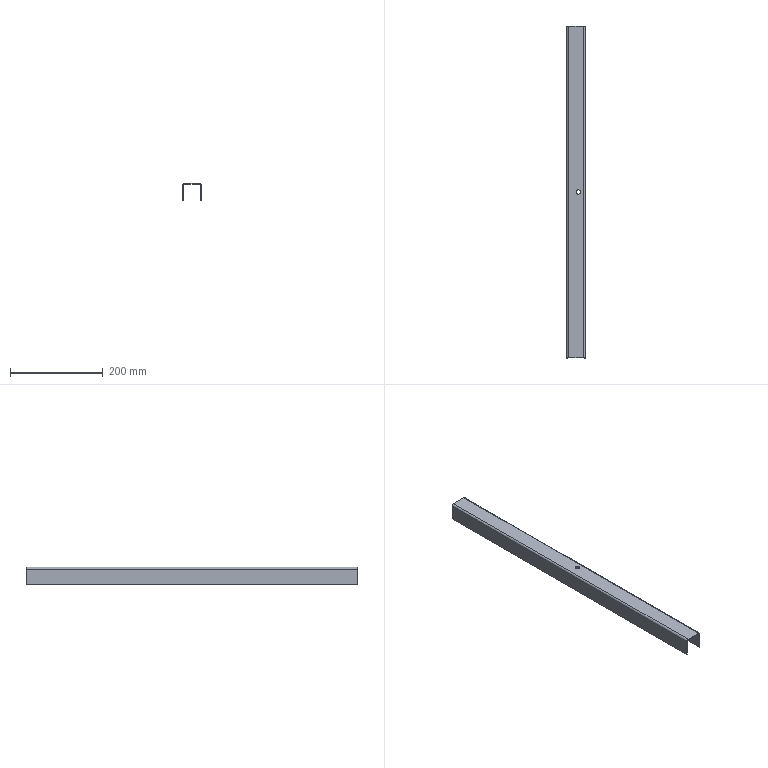Part | NX | features solid 2 | 1 solid | 16 faces | box 40 x 717 x 38 mm | volume 156782 mm3 | plane 10 | cylinder 6 | commonest cylinder face diameters 4 x2 8 x2 9.2 x2
STEP:
#1=CARTESIAN_POINT('',(-836.,-1113.1,1293.));
#2=VERTEX_POINT('',#1);
#3=CARTESIAN_POINT('',(-836.,-1113.1,1295.));
#4=VERTEX_POINT('',#3);
#5=CARTESIAN_POINT('',(-836.,-1113.1,575.88));
#6=DIRECTION('',(0.,0.,1.));
#7=VECTOR('',#6,1000.);
#8=LINE('',#5,#7);
#9=EDGE_CURVE('',#2,#4,#8,.T.);
#10=ORIENTED_EDGE('',*,*,#9,.F.);
#11=CARTESIAN_POINT('',(-836.,-1103.9,1293.));
#12=VERTEX_POINT('',#11);
#13=CARTESIAN_POINT('',(-836.,-1108.5,1293.));
#14=DIRECTION('',(0.,0.,-1.));
#15=DIRECTION('',(0.,-1.,0.));
#16=AXIS2_PLACEMENT_3D('',#13,#14,#15);
#17=CIRCLE('',#16,4.6);
#18=EDGE_CURVE('',#2,#12,#17,.T.);
#19=ORIENTED_EDGE('',*,*,#18,.T.);
#20=CARTESIAN_POINT('',(-836.,-1103.9,1295.));
#21=VERTEX_POINT('',#20);
#22=CARTESIAN_POINT('',(-836.,-1103.9,575.88));
#23=DIRECTION('',(0.,0.,1.));
#24=VECTOR('',#23,1000.);
#25=LINE('',#22,#24);
#26=EDGE_CURVE('',#21,#12,#25,.F.);
#27=ORIENTED_EDGE('',*,*,#26,.F.);
#28=CARTESIAN_POINT('',(-836.,-1108.5,1295.));
#29=DIRECTION('',(0.,0.,1.));
#30=DIRECTION('',(0.,-1.,0.));
#31=AXIS2_PLACEMENT_3D('',#28,#29,#30);
#32=CIRCLE('',#31,4.6);
#33=EDGE_CURVE('',#21,#4,#32,.T.);
#34=ORIENTED_EDGE('',*,*,#33,.T.);
#35=EDGE_LOOP('',(#10,#19,#27,#34));
#36=FACE_BOUND('',#35,.T.);
#37=CARTESIAN_POINT('',(-836.,-1108.5,575.88));
#38=DIRECTION('',(0.,0.,1.));
#39=DIRECTION('',(0.,1.,0.));
#40=AXIS2_PLACEMENT_3D('',#37,#38,#39);
#41=CYLINDRICAL_SURFACE('',#40,4.6);
#42=ADVANCED_FACE('',(#36),#41,.F.);
#43=CARTESIAN_POINT('',(-821.,-1467.,1291.));
#44=VERTEX_POINT('',#43);
#45=CARTESIAN_POINT('',(-821.,-1467.,1257.));
#46=VERTEX_POINT('',#45);
#47=CARTESIAN_POINT('',(-821.,-1467.,1295.));
#48=DIRECTION('',(0.,0.,-1.));
#49=VECTOR('',#48,1000.);
#50=LINE('',#47,#49);
#51=EDGE_CURVE('',#44,#46,#50,.T.);
#52=ORIENTED_EDGE('',*,*,#51,.T.);
#53=CARTESIAN_POINT('',(-821.,-750.,1257.));
#54=VERTEX_POINT('',#53);
#55=CARTESIAN_POINT('',(-821.,-750.,1257.));
#56=DIRECTION('',(0.,-1.,0.));
#57=VECTOR('',#56,1000.);
#58=LINE('',#55,#57);
#59=EDGE_CURVE('',#54,#46,#58,.T.);
#60=ORIENTED_EDGE('',*,*,#59,.F.);
#61=CARTESIAN_POINT('',(-821.,-750.,1291.));
#62=VERTEX_POINT('',#61);
#63=CARTESIAN_POINT('',(-821.,-750.,1295.));
#64=DIRECTION('',(0.,0.,-1.));
#65=VECTOR('',#64,1000.);
#66=LINE('',#63,#65);
#67=EDGE_CURVE('',#62,#54,#66,.T.);
#68=ORIENTED_EDGE('',*,*,#67,.F.);
#69=CARTESIAN_POINT('',(-821.,-750.,1291.));
#70=DIRECTION('',(0.,-1.,0.));
#71=VECTOR('',#70,1000.);
#72=LINE('',#69,#71);
#73=EDGE_CURVE('',#62,#44,#72,.T.);
#74=ORIENTED_EDGE('',*,*,#73,.T.);
#75=EDGE_LOOP('',(#52,#60,#68,#74));
#76=FACE_BOUND('',#75,.T.);
#77=CARTESIAN_POINT('',(-821.,-750.,1295.));
#78=DIRECTION('',(-1.,0.,0.));
#79=DIRECTION('',(0.,0.,1.));
#80=AXIS2_PLACEMENT_3D('',#77,#78,#79);
#81=PLANE('',#80);
#82=ADVANCED_FACE('',(#76),#81,.F.);
#83=CARTESIAN_POINT('',(-825.,-1467.,1295.));
#84=VERTEX_POINT('',#83);
#85=CARTESIAN_POINT('',(-825.,-1467.,1291.));
#86=DIRECTION('',(0.,1.,0.));
#87=DIRECTION('',(-1.,0.,0.));
#88=AXIS2_PLACEMENT_3D('',#85,#86,#87);
#89=CIRCLE('',#88,4.);
#90=EDGE_CURVE('',#84,#44,#89,.T.);
#91=ORIENTED_EDGE('',*,*,#90,.T.);
#92=ORIENTED_EDGE('',*,*,#73,.F.);
#93=CARTESIAN_POINT('',(-825.,-750.,1295.));
#94=VERTEX_POINT('',#93);
#95=CARTESIAN_POINT('',(-825.,-750.,1291.));
#96=DIRECTION('',(0.,1.,0.));
#97=DIRECTION('',(-1.,0.,0.));
#98=AXIS2_PLACEMENT_3D('',#95,#96,#97);
#99=CIRCLE('',#98,4.);
#100=EDGE_CURVE('',#94,#62,#99,.T.);
#101=ORIENTED_EDGE('',*,*,#100,.F.);
#102=CARTESIAN_POINT('',(-825.,-750.,1295.));
#103=DIRECTION('',(0.,-1.,0.));
#104=VECTOR('',#103,1000.);
#105=LINE('',#102,#104);
#106=EDGE_CURVE('',#94,#84,#105,.T.);
#107=ORIENTED_EDGE('',*,*,#106,.T.);
#108=EDGE_LOOP('',(#91,#92,#101,#107));
#109=FACE_BOUND('',#108,.T.);
#110=CARTESIAN_POINT('',(-825.,-750.,1291.));
#111=DIRECTION('',(0.,-1.,0.));
#112=DIRECTION('',(0.,0.,1.));
#113=AXIS2_PLACEMENT_3D('',#110,#111,#112);
#114=CYLINDRICAL_SURFACE('',#113,4.);
#115=ADVANCED_FACE('',(#109),#114,.T.);
#116=ORIENTED_EDGE('',*,*,#33,.F.);
#117=CARTESIAN_POINT('',(-836.,-1108.5,1295.));
#118=DIRECTION('',(0.,0.,1.));
#119=DIRECTION('',(0.,-1.,0.));
#120=AXIS2_PLACEMENT_3D('',#117,#118,#119);
#121=CIRCLE('',#120,4.6);
#122=EDGE_CURVE('',#4,#21,#121,.T.);
#123=ORIENTED_EDGE('',*,*,#122,.F.);
#124=EDGE_LOOP('',(#116,#123));
#125=FACE_BOUND('',#124,.T.);
#126=CARTESIAN_POINT('',(-857.,-1467.,1295.));
#127=VERTEX_POINT('',#126);
#128=CARTESIAN_POINT('',(-861.,-1467.,1295.));
#129=DIRECTION('',(1.,0.,0.));
#130=VECTOR('',#129,1000.);
#131=LINE('',#128,#130);
#132=EDGE_CURVE('',#127,#84,#131,.T.);
#133=ORIENTED_EDGE('',*,*,#132,.T.);
#134=ORIENTED_EDGE('',*,*,#106,.F.);
#135=CARTESIAN_POINT('',(-857.,-750.,1295.));
#136=VERTEX_POINT('',#135);
#137=CARTESIAN_POINT('',(-861.,-750.,1295.));
#138=DIRECTION('',(1.,0.,0.));
#139=VECTOR('',#138,1000.);
#140=LINE('',#137,#139);
#141=EDGE_CURVE('',#136,#94,#140,.T.);
#142=ORIENTED_EDGE('',*,*,#141,.F.);
#143=CARTESIAN_POINT('',(-857.,-750.,1295.));
#144=DIRECTION('',(0.,-1.,0.));
#145=VECTOR('',#144,1000.);
#146=LINE('',#143,#145);
#147=EDGE_CURVE('',#136,#127,#146,.T.);
#148=ORIENTED_EDGE('',*,*,#147,.T.);
#149=EDGE_LOOP('',(#133,#134,#142,#148));
#150=FACE_BOUND('',#149,.T.);
#151=CARTESIAN_POINT('',(-861.,-750.,1295.));
#152=DIRECTION('',(0.,0.,-1.));
#153=DIRECTION('',(0.,-1.,0.));
#154=AXIS2_PLACEMENT_3D('',#151,#152,#153);
#155=PLANE('',#154);
#156=ADVANCED_FACE('',(#125,#150),#155,.F.);
#157=CARTESIAN_POINT('',(-861.,-1467.,1291.));
#158=VERTEX_POINT('',#157);
#159=CARTESIAN_POINT('',(-857.,-1467.,1291.));
#160=DIRECTION('',(0.,1.,0.));
#161=DIRECTION('',(-1.,0.,0.));
#162=AXIS2_PLACEMENT_3D('',#159,#160,#161);
#163=CIRCLE('',#162,4.);
#164=EDGE_CURVE('',#158,#127,#163,.T.);
#165=ORIENTED_EDGE('',*,*,#164,.T.);
#166=ORIENTED_EDGE('',*,*,#147,.F.);
#167=CARTESIAN_POINT('',(-861.,-750.,1291.));
#168=VERTEX_POINT('',#167);
#169=CARTESIAN_POINT('',(-857.,-750.,1291.));
#170=DIRECTION('',(0.,1.,0.));
#171=DIRECTION('',(-1.,0.,0.));
#172=AXIS2_PLACEMENT_3D('',#169,#170,#171);
#173=CIRCLE('',#172,4.);
#174=EDGE_CURVE('',#168,#136,#173,.T.);
#175=ORIENTED_EDGE('',*,*,#174,.F.);
#176=CARTESIAN_POINT('',(-861.,-750.,1291.));
#177=DIRECTION('',(0.,-1.,0.));
#178=VECTOR('',#177,1000.);
#179=LINE('',#176,#178);
#180=EDGE_CURVE('',#168,#158,#179,.T.);
#181=ORIENTED_EDGE('',*,*,#180,.T.);
#182=EDGE_LOOP('',(#165,#166,#175,#181));
#183=FACE_BOUND('',#182,.T.);
#184=CARTESIAN_POINT('',(-857.,-750.,1291.));
#185=DIRECTION('',(0.,-1.,0.));
#186=DIRECTION('',(0.,0.,1.));
#187=AXIS2_PLACEMENT_3D('',#184,#185,#186);
#188=CYLINDRICAL_SURFACE('',#187,4.);
#189=ADVANCED_FACE('',(#183),#188,.T.);
#190=CARTESIAN_POINT('',(-861.,-1467.,1257.));
#191=VERTEX_POINT('',#190);
#192=CARTESIAN_POINT('',(-861.,-1467.,1257.));
#193=DIRECTION('',(0.,0.,1.));
#194=VECTOR('',#193,1000.);
#195=LINE('',#192,#194);
#196=EDGE_CURVE('',#191,#158,#195,.T.);
#197=ORIENTED_EDGE('',*,*,#196,.T.);
#198=ORIENTED_EDGE('',*,*,#180,.F.);
#199=CARTESIAN_POINT('',(-861.,-750.,1257.));
#200=VERTEX_POINT('',#199);
#201=CARTESIAN_POINT('',(-861.,-750.,1257.));
#202=DIRECTION('',(0.,0.,1.));
#203=VECTOR('',#202,1000.);
#204=LINE('',#201,#203);
#205=EDGE_CURVE('',#200,#168,#204,.T.);
#206=ORIENTED_EDGE('',*,*,#205,.F.);
#207=CARTESIAN_POINT('',(-861.,-750.,1257.));
#208=DIRECTION('',(0.,-1.,0.));
#209=VECTOR('',#208,1000.);
#210=LINE('',#207,#209);
#211=EDGE_CURVE('',#200,#191,#210,.T.);
#212=ORIENTED_EDGE('',*,*,#211,.T.);
#213=EDGE_LOOP('',(#197,#198,#206,#212));
#214=FACE_BOUND('',#213,.T.);
#215=CARTESIAN_POINT('',(-861.,-750.,1257.));
#216=DIRECTION('',(1.,0.,0.));
#217=DIRECTION('',(0.,0.,1.));
#218=AXIS2_PLACEMENT_3D('',#215,#216,#217);
#219=PLANE('',#218);
#220=ADVANCED_FACE('',(#214),#219,.F.);
#221=CARTESIAN_POINT('',(-823.,-1467.,1291.));
#222=VERTEX_POINT('',#221);
#223=CARTESIAN_POINT('',(-823.,-1467.,1257.));
#224=VERTEX_POINT('',#223);
#225=CARTESIAN_POINT('',(-823.,-1467.,1295.));
#226=DIRECTION('',(0.,0.,-1.));
#227=VECTOR('',#226,1000.);
#228=LINE('',#225,#227);
#229=EDGE_CURVE('',#222,#224,#228,.T.);
#230=ORIENTED_EDGE('',*,*,#229,.F.);
#231=CARTESIAN_POINT('',(-823.,-750.,1291.));
#232=VERTEX_POINT('',#231);
#233=CARTESIAN_POINT('',(-823.,-750.,1291.));
#234=DIRECTION('',(0.,-1.,0.));
#235=VECTOR('',#234,1000.);
#236=LINE('',#233,#235);
#237=EDGE_CURVE('',#232,#222,#236,.T.);
#238=ORIENTED_EDGE('',*,*,#237,.F.);
#239=CARTESIAN_POINT('',(-823.,-750.,1257.));
#240=VERTEX_POINT('',#239);
#241=CARTESIAN_POINT('',(-823.,-750.,1295.));
#242=DIRECTION('',(0.,0.,-1.));
#243=VECTOR('',#242,1000.);
#244=LINE('',#241,#243);
#245=EDGE_CURVE('',#232,#240,#244,.T.);
#246=ORIENTED_EDGE('',*,*,#245,.T.);
#247=CARTESIAN_POINT('',(-823.,-750.,1257.));
#248=DIRECTION('',(0.,-1.,0.));
#249=VECTOR('',#248,1000.);
#250=LINE('',#247,#249);
#251=EDGE_CURVE('',#240,#224,#250,.T.);
#252=ORIENTED_EDGE('',*,*,#251,.T.);
#253=EDGE_LOOP('',(#230,#238,#246,#252));
#254=FACE_BOUND('',#253,.T.);
#255=CARTESIAN_POINT('',(-823.,-750.,1295.));
#256=DIRECTION('',(-1.,0.,0.));
#257=DIRECTION('',(0.,0.,1.));
#258=AXIS2_PLACEMENT_3D('',#255,#256,#257);
#259=PLANE('',#258);
#260=ADVANCED_FACE('',(#254),#259,.T.);
#261=CARTESIAN_POINT('',(-825.,-1467.,1293.));
#262=VERTEX_POINT('',#261);
#263=CARTESIAN_POINT('',(-825.,-1467.,1291.));
#264=DIRECTION('',(0.,1.,0.));
#265=DIRECTION('',(0.,0.,1.));
#266=AXIS2_PLACEMENT_3D('',#263,#264,#265);
#267=CIRCLE('',#266,2.);
#268=EDGE_CURVE('',#262,#222,#267,.T.);
#269=ORIENTED_EDGE('',*,*,#268,.F.);
#270=CARTESIAN_POINT('',(-825.,-750.,1293.));
#271=VERTEX_POINT('',#270);
#272=CARTESIAN_POINT('',(-825.,-750.,1293.));
#273=DIRECTION('',(0.,-1.,0.));
#274=VECTOR('',#273,1000.);
#275=LINE('',#272,#274);
#276=EDGE_CURVE('',#271,#262,#275,.T.);
#277=ORIENTED_EDGE('',*,*,#276,.F.);
#278=CARTESIAN_POINT('',(-825.,-750.,1291.));
#279=DIRECTION('',(0.,1.,0.));
#280=DIRECTION('',(0.,0.,1.));
#281=AXIS2_PLACEMENT_3D('',#278,#279,#280);
#282=CIRCLE('',#281,2.);
#283=EDGE_CURVE('',#271,#232,#282,.T.);
#284=ORIENTED_EDGE('',*,*,#283,.T.);
#285=ORIENTED_EDGE('',*,*,#237,.T.);
#286=EDGE_LOOP('',(#269,#277,#284,#285));
#287=FACE_BOUND('',#286,.T.);
#288=CARTESIAN_POINT('',(-825.,-750.,1291.));
#289=DIRECTION('',(0.,-1.,0.));
#290=DIRECTION('',(0.,0.,1.));
#291=AXIS2_PLACEMENT_3D('',#288,#289,#290);
#292=CYLINDRICAL_SURFACE('',#291,2.);
#293=ADVANCED_FACE('',(#287),#292,.F.);
#294=CARTESIAN_POINT('',(-836.,-1108.5,1293.));
#295=DIRECTION('',(0.,0.,-1.));
#296=DIRECTION('',(0.,-1.,0.));
#297=AXIS2_PLACEMENT_3D('',#294,#295,#296);
#298=CIRCLE('',#297,4.6);
#299=EDGE_CURVE('',#12,#2,#298,.T.);
#300=ORIENTED_EDGE('',*,*,#299,.F.);
#301=ORIENTED_EDGE('',*,*,#18,.F.);
#302=EDGE_LOOP('',(#300,#301));
#303=FACE_BOUND('',#302,.T.);
#304=CARTESIAN_POINT('',(-857.,-1467.,1293.));
#305=VERTEX_POINT('',#304);
#306=CARTESIAN_POINT('',(-861.,-1467.,1293.));
#307=DIRECTION('',(1.,0.,0.));
#308=VECTOR('',#307,1000.);
#309=LINE('',#306,#308);
#310=EDGE_CURVE('',#305,#262,#309,.T.);
#311=ORIENTED_EDGE('',*,*,#310,.F.);
#312=CARTESIAN_POINT('',(-857.,-750.,1293.));
#313=VERTEX_POINT('',#312);
#314=CARTESIAN_POINT('',(-857.,-750.,1293.));
#315=DIRECTION('',(0.,-1.,0.));
#316=VECTOR('',#315,1000.);
#317=LINE('',#314,#316);
#318=EDGE_CURVE('',#313,#305,#317,.T.);
#319=ORIENTED_EDGE('',*,*,#318,.F.);
#320=CARTESIAN_POINT('',(-861.,-750.,1293.));
#321=DIRECTION('',(1.,0.,0.));
#322=VECTOR('',#321,1000.);
#323=LINE('',#320,#322);
#324=EDGE_CURVE('',#313,#271,#323,.T.);
#325=ORIENTED_EDGE('',*,*,#324,.T.);
#326=ORIENTED_EDGE('',*,*,#276,.T.);
#327=EDGE_LOOP('',(#311,#319,#325,#326));
#328=FACE_BOUND('',#327,.T.);
#329=CARTESIAN_POINT('',(-861.,-750.,1293.));
#330=DIRECTION('',(0.,0.,-1.));
#331=DIRECTION('',(0.,-1.,0.));
#332=AXIS2_PLACEMENT_3D('',#329,#330,#331);
#333=PLANE('',#332);
#334=ADVANCED_FACE('',(#303,#328),#333,.T.);
#335=CARTESIAN_POINT('',(-859.,-1467.,1291.));
#336=VERTEX_POINT('',#335);
#337=CARTESIAN_POINT('',(-857.,-1467.,1291.));
#338=DIRECTION('',(0.,1.,0.));
#339=DIRECTION('',(0.,0.,1.));
#340=AXIS2_PLACEMENT_3D('',#337,#338,#339);
#341=CIRCLE('',#340,2.);
#342=EDGE_CURVE('',#336,#305,#341,.T.);
#343=ORIENTED_EDGE('',*,*,#342,.F.);
#344=CARTESIAN_POINT('',(-859.,-750.,1291.));
#345=VERTEX_POINT('',#344);
#346=CARTESIAN_POINT('',(-859.,-750.,1291.));
#347=DIRECTION('',(0.,-1.,0.));
#348=VECTOR('',#347,1000.);
#349=LINE('',#346,#348);
#350=EDGE_CURVE('',#345,#336,#349,.T.);
#351=ORIENTED_EDGE('',*,*,#350,.F.);
#352=CARTESIAN_POINT('',(-857.,-750.,1291.));
#353=DIRECTION('',(0.,1.,0.));
#354=DIRECTION('',(0.,0.,1.));
#355=AXIS2_PLACEMENT_3D('',#352,#353,#354);
#356=CIRCLE('',#355,2.);
#357=EDGE_CURVE('',#345,#313,#356,.T.);
#358=ORIENTED_EDGE('',*,*,#357,.T.);
#359=ORIENTED_EDGE('',*,*,#318,.T.);
#360=EDGE_LOOP('',(#343,#351,#358,#359));
#361=FACE_BOUND('',#360,.T.);
#362=CARTESIAN_POINT('',(-857.,-750.,1291.));
#363=DIRECTION('',(0.,-1.,0.));
#364=DIRECTION('',(0.,0.,1.));
#365=AXIS2_PLACEMENT_3D('',#362,#363,#364);
#366=CYLINDRICAL_SURFACE('',#365,2.);
#367=ADVANCED_FACE('',(#361),#366,.F.);
#368=CARTESIAN_POINT('',(-859.,-1467.,1257.));
#369=VERTEX_POINT('',#368);
#370=CARTESIAN_POINT('',(-859.,-1467.,1257.));
#371=DIRECTION('',(0.,0.,1.));
#372=VECTOR('',#371,1000.);
#373=LINE('',#370,#372);
#374=EDGE_CURVE('',#369,#336,#373,.T.);
#375=ORIENTED_EDGE('',*,*,#374,.F.);
#376=CARTESIAN_POINT('',(-859.,-750.,1257.));
#377=VERTEX_POINT('',#376);
#378=CARTESIAN_POINT('',(-859.,-750.,1257.));
#379=DIRECTION('',(0.,-1.,0.));
#380=VECTOR('',#379,1000.);
#381=LINE('',#378,#380);
#382=EDGE_CURVE('',#377,#369,#381,.T.);
#383=ORIENTED_EDGE('',*,*,#382,.F.);
#384=CARTESIAN_POINT('',(-859.,-750.,1257.));
#385=DIRECTION('',(0.,0.,1.));
#386=VECTOR('',#385,1000.);
#387=LINE('',#384,#386);
#388=EDGE_CURVE('',#377,#345,#387,.T.);
#389=ORIENTED_EDGE('',*,*,#388,.T.);
#390=ORIENTED_EDGE('',*,*,#350,.T.);
#391=EDGE_LOOP('',(#375,#383,#389,#390));
#392=FACE_BOUND('',#391,.T.);
#393=CARTESIAN_POINT('',(-859.,-750.,1257.));
#394=DIRECTION('',(1.,0.,0.));
#395=DIRECTION('',(0.,0.,1.));
#396=AXIS2_PLACEMENT_3D('',#393,#394,#395);
#397=PLANE('',#396);
#398=ADVANCED_FACE('',(#392),#397,.T.);
#399=ORIENTED_EDGE('',*,*,#211,.F.);
#400=CARTESIAN_POINT('',(-861.,-750.,1257.));
#401=DIRECTION('',(1.,0.,0.));
#402=VECTOR('',#401,1000.);
#403=LINE('',#400,#402);
#404=EDGE_CURVE('',#200,#377,#403,.T.);
#405=ORIENTED_EDGE('',*,*,#404,.T.);
#406=ORIENTED_EDGE('',*,*,#382,.T.);
#407=CARTESIAN_POINT('',(-861.,-1467.,1257.));
#408=DIRECTION('',(1.,0.,0.));
#409=VECTOR('',#408,1000.);
#410=LINE('',#407,#409);
#411=EDGE_CURVE('',#191,#369,#410,.T.);
#412=ORIENTED_EDGE('',*,*,#411,.F.);
#413=EDGE_LOOP('',(#399,#405,#406,#412));
#414=FACE_BOUND('',#413,.T.);
#415=CARTESIAN_POINT('',(-861.,-750.,1257.));
#416=DIRECTION('',(0.,0.,1.));
#417=DIRECTION('',(1.,0.,0.));
#418=AXIS2_PLACEMENT_3D('',#415,#416,#417);
#419=PLANE('',#418);
#420=ADVANCED_FACE('',(#414),#419,.F.);
#421=ORIENTED_EDGE('',*,*,#374,.T.);
#422=ORIENTED_EDGE('',*,*,#342,.T.);
#423=ORIENTED_EDGE('',*,*,#310,.T.);
#424=ORIENTED_EDGE('',*,*,#268,.T.);
#425=ORIENTED_EDGE('',*,*,#229,.T.);
#426=CARTESIAN_POINT('',(-821.,-1467.,1257.));
#427=DIRECTION('',(-1.,0.,0.));
#428=VECTOR('',#427,1000.);
#429=LINE('',#426,#428);
#430=EDGE_CURVE('',#46,#224,#429,.T.);
#431=ORIENTED_EDGE('',*,*,#430,.F.);
#432=ORIENTED_EDGE('',*,*,#51,.F.);
#433=ORIENTED_EDGE('',*,*,#90,.F.);
#434=ORIENTED_EDGE('',*,*,#132,.F.);
#435=ORIENTED_EDGE('',*,*,#164,.F.);
#436=ORIENTED_EDGE('',*,*,#196,.F.);
#437=ORIENTED_EDGE('',*,*,#411,.T.);
#438=EDGE_LOOP('',(#421,#422,#423,#424,#425,#431,#432,#433,#434,#435,#436,#437));
#439=FACE_BOUND('',#438,.T.);
#440=CARTESIAN_POINT('',(-861.,-1467.,1257.));
#441=DIRECTION('',(0.,1.,0.));
#442=DIRECTION('',(0.,0.,-1.));
#443=AXIS2_PLACEMENT_3D('',#440,#441,#442);
#444=PLANE('',#443);
#445=ADVANCED_FACE('',(#439),#444,.F.);
#446=CARTESIAN_POINT('',(-821.,-750.,1257.));
#447=DIRECTION('',(-1.,0.,0.));
#448=VECTOR('',#447,1000.);
#449=LINE('',#446,#448);
#450=EDGE_CURVE('',#54,#240,#449,.T.);
#451=ORIENTED_EDGE('',*,*,#450,.F.);
#452=ORIENTED_EDGE('',*,*,#59,.T.);
#453=ORIENTED_EDGE('',*,*,#430,.T.);
#454=ORIENTED_EDGE('',*,*,#251,.F.);
#455=EDGE_LOOP('',(#451,#452,#453,#454));
#456=FACE_BOUND('',#455,.T.);
#457=CARTESIAN_POINT('',(-821.,-750.,1257.));
#458=DIRECTION('',(0.,0.,-1.));
#459=DIRECTION('',(0.,-1.,0.));
#460=AXIS2_PLACEMENT_3D('',#457,#458,#459);
#461=PLANE('',#460);
#462=ADVANCED_FACE('',(#456),#461,.T.);
#463=ORIENTED_EDGE('',*,*,#245,.F.);
#464=ORIENTED_EDGE('',*,*,#283,.F.);
#465=ORIENTED_EDGE('',*,*,#324,.F.);
#466=ORIENTED_EDGE('',*,*,#357,.F.);
#467=ORIENTED_EDGE('',*,*,#388,.F.);
#468=ORIENTED_EDGE('',*,*,#404,.F.);
#469=ORIENTED_EDGE('',*,*,#205,.T.);
#470=ORIENTED_EDGE('',*,*,#174,.T.);
#471=ORIENTED_EDGE('',*,*,#141,.T.);
#472=ORIENTED_EDGE('',*,*,#100,.T.);
#473=ORIENTED_EDGE('',*,*,#67,.T.);
#474=ORIENTED_EDGE('',*,*,#450,.T.);
#475=EDGE_LOOP('',(#463,#464,#465,#466,#467,#468,#469,#470,#471,#472,#473,#474));
#476=FACE_BOUND('',#475,.T.);
#477=CARTESIAN_POINT('',(-821.,-750.,1295.));
#478=DIRECTION('',(0.,1.,0.));
#479=DIRECTION('',(0.,0.,-1.));
#480=AXIS2_PLACEMENT_3D('',#477,#478,#479);
#481=PLANE('',#480);
#482=ADVANCED_FACE('',(#476),#481,.T.);
#483=ORIENTED_EDGE('',*,*,#299,.T.);
#484=ORIENTED_EDGE('',*,*,#9,.T.);
#485=ORIENTED_EDGE('',*,*,#122,.T.);
#486=ORIENTED_EDGE('',*,*,#26,.T.);
#487=EDGE_LOOP('',(#483,#484,#485,#486));
#488=FACE_BOUND('',#487,.T.);
#489=CARTESIAN_POINT('',(-836.,-1108.5,575.88));
#490=DIRECTION('',(0.,0.,1.));
#491=DIRECTION('',(0.,1.,0.));
#492=AXIS2_PLACEMENT_3D('',#489,#490,#491);
#493=CYLINDRICAL_SURFACE('',#492,4.6);
#494=ADVANCED_FACE('',(#488),#493,.F.);
#495=CLOSED_SHELL('',(#42,#82,#115,#156,#189,#220,#260,#293,#334,#367,#398,#420,#445,#462,#482,#494));
#496=MANIFOLD_SOLID_BREP('',#495);
#497=(LENGTH_UNIT()NAMED_UNIT(*)SI_UNIT(.MILLI.,.METRE.));
#498=UNCERTAINTY_MEASURE_WITH_UNIT(LENGTH_MEASURE(0.00001),#497,'','');
#499=(NAMED_UNIT(*)PLANE_ANGLE_UNIT()SI_UNIT($,.RADIAN.));
#500=(NAMED_UNIT(*)SI_UNIT($,.STERADIAN.)SOLID_ANGLE_UNIT());
#501=(GEOMETRIC_REPRESENTATION_CONTEXT(3)GLOBAL_UNCERTAINTY_ASSIGNED_CONTEXT((#498))GLOBAL_UNIT_ASSIGNED_CONTEXT((#497,#499,#500))REPRESENTATION_CONTEXT('',''));
#502=ADVANCED_BREP_SHAPE_REPRESENTATION('',(#496),#501);